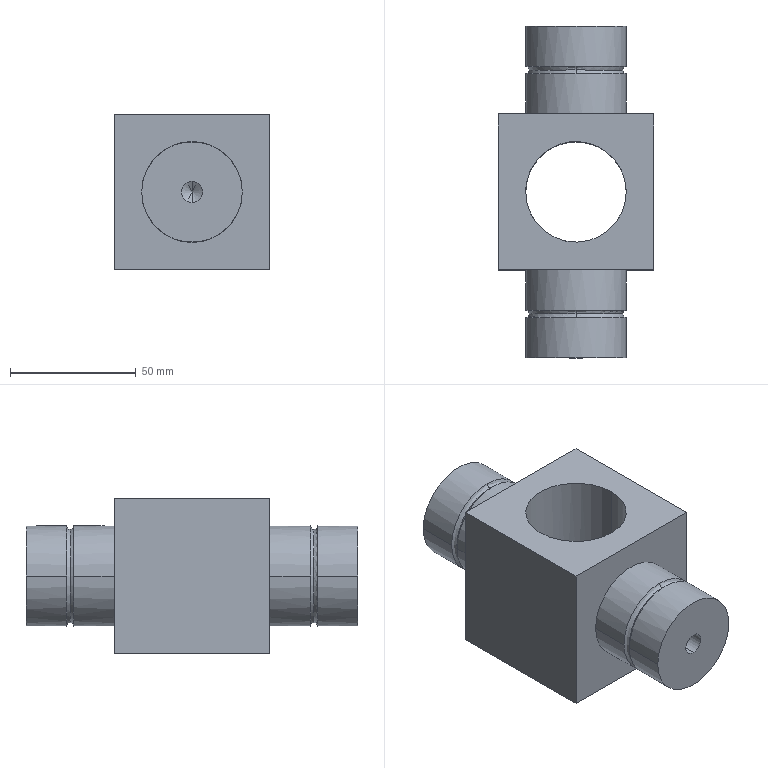Part | STEP file | LM-05-1238 | 1 solid | 34 faces | box 62 x 132 x 62 mm | volume 244471 mm3 | spline 24 | cylinder 6 | cone 4 | commonest cylinder face diameters 8.5 x4 40 x2